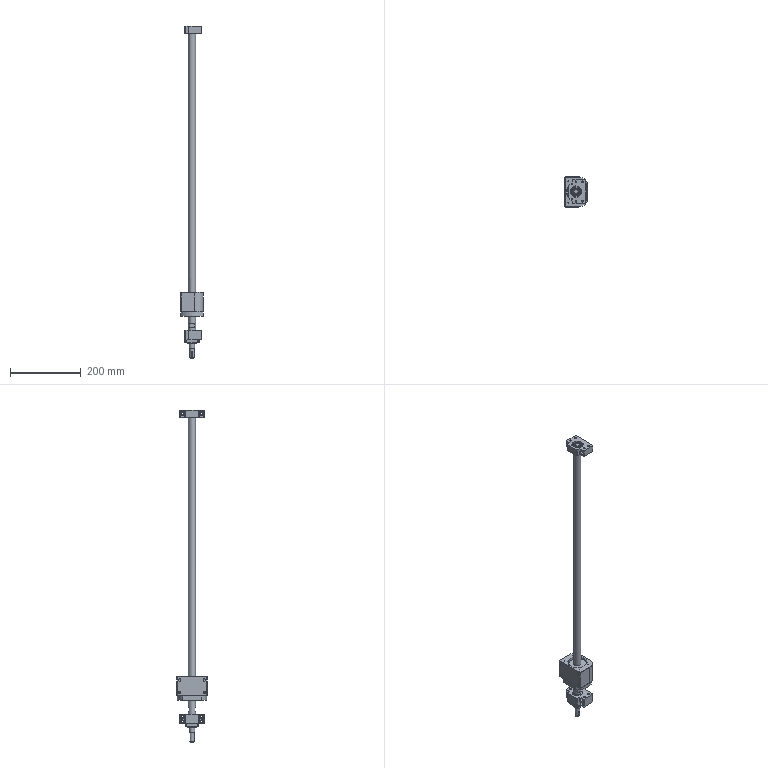Part | NX | 3 solids | 274 faces | box 64 x 85 x 937.495 mm | volume 705358 mm3 | plane 140 | cylinder 91 | cone 36 | spline 5 | torus 2 | commonest cylinder face diameters 5.5 x16 6.6 x10 6.8 x8 11 x6 15 x6 50 x6